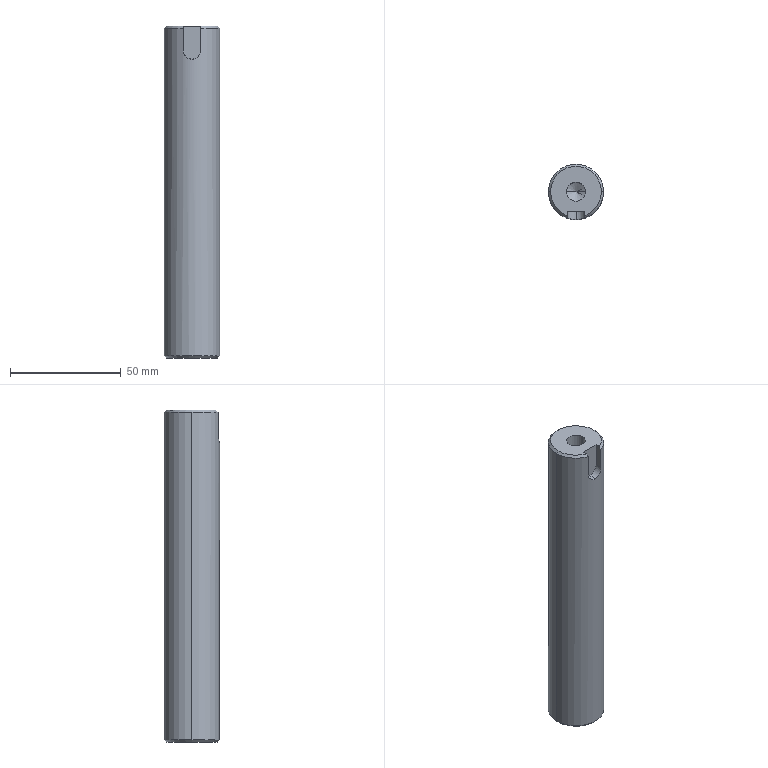Part | SolidWorks | features Chamfer 1, Extrusion 1, Fillet 1, HoleWzd 1, ICE 1 | 1 solid | 18 faces | box 25 x 25 x 150 mm | volume 71725 mm3 | cone 7 | cylinder 6 | plane 5 | commonest cylinder face diameters 8 x2 8.5 x2 25 x2
STEP:
#1=CARTESIAN_POINT('',(-4.25,0.,50.5));
#2=VERTEX_POINT('',#1);
#3=CARTESIAN_POINT('',(4.25,0.,50.5));
#4=VERTEX_POINT('',#3);
#5=CARTESIAN_POINT('',(0.,0.,50.5));
#6=DIRECTION('',(0.,0.,1.));
#7=DIRECTION('',(1.,0.,0.));
#8=AXIS2_PLACEMENT_3D('',#5,#6,#7);
#9=CIRCLE('',#8,4.25);
#10=EDGE_CURVE('',#2,#4,#9,.T.);
#11=ORIENTED_EDGE('',*,*,#10,.F.);
#12=CARTESIAN_POINT('',(-4.25,0.,75.));
#13=VERTEX_POINT('',#12);
#14=CARTESIAN_POINT('',(-4.25,0.,75.));
#15=DIRECTION('',(0.,0.,1.));
#16=VECTOR('',#15,1000.);
#17=LINE('',#14,#16);
#18=EDGE_CURVE('',#2,#13,#17,.T.);
#19=ORIENTED_EDGE('',*,*,#18,.T.);
#20=CARTESIAN_POINT('',(4.25,0.,75.));
#21=VERTEX_POINT('',#20);
#22=CARTESIAN_POINT('',(0.,0.,75.));
#23=DIRECTION('',(0.,0.,1.));
#24=DIRECTION('',(1.,0.,0.));
#25=AXIS2_PLACEMENT_3D('',#22,#23,#24);
#26=CIRCLE('',#25,4.25);
#27=EDGE_CURVE('',#13,#21,#26,.T.);
#28=ORIENTED_EDGE('',*,*,#27,.T.);
#29=CARTESIAN_POINT('',(4.25,0.,75.));
#30=DIRECTION('',(0.,0.,1.));
#31=VECTOR('',#30,1000.);
#32=LINE('',#29,#31);
#33=EDGE_CURVE('',#4,#21,#32,.T.);
#34=ORIENTED_EDGE('',*,*,#33,.F.);
#35=EDGE_LOOP('',(#11,#19,#28,#34));
#36=FACE_OUTER_BOUND('',#35,.T.);
#37=CARTESIAN_POINT('',(0.,0.,75.));
#38=DIRECTION('',(0.,0.,1.));
#39=DIRECTION('',(1.,0.,0.));
#40=AXIS2_PLACEMENT_3D('',#37,#38,#39);
#41=CYLINDRICAL_SURFACE('',#40,4.25);
#42=ADVANCED_FACE('',(#36),#41,.F.);
#43=CARTESIAN_POINT('',(0.,0.,47.946));
#44=VERTEX_POINT('',#43);
#45=CARTESIAN_POINT('',(4.25,0.,50.5));
#46=DIRECTION('',(0.8572,0.,0.515));
#47=VECTOR('',#46,1000.);
#48=LINE('',#45,#47);
#49=EDGE_CURVE('',#44,#4,#48,.T.);
#50=ORIENTED_EDGE('',*,*,#49,.F.);
#51=CARTESIAN_POINT('',(-4.25,0.,50.5));
#52=DIRECTION('',(-0.8572,0.,0.515));
#53=VECTOR('',#52,1000.);
#54=LINE('',#51,#53);
#55=EDGE_CURVE('',#44,#2,#54,.T.);
#56=ORIENTED_EDGE('',*,*,#55,.T.);
#57=ORIENTED_EDGE('',*,*,#10,.T.);
#58=EDGE_LOOP('',(#50,#56,#57));
#59=FACE_OUTER_BOUND('',#58,.T.);
#60=CARTESIAN_POINT('',(0.,0.,50.5));
#61=DIRECTION('',(0.,0.,1.));
#62=DIRECTION('',(1.,0.,0.));
#63=AXIS2_PLACEMENT_3D('',#60,#61,#62);
#64=CONICAL_SURFACE('',#63,4.25,1.03);
#65=ADVANCED_FACE('',(#59),#64,.F.);
#66=CARTESIAN_POINT('',(11.5,0.,75.));
#67=VERTEX_POINT('',#66);
#68=CARTESIAN_POINT('',(-11.5,0.,75.));
#69=VERTEX_POINT('',#68);
#70=CARTESIAN_POINT('',(0.,0.,75.));
#71=DIRECTION('',(0.,0.,1.));
#72=DIRECTION('',(1.,0.,0.));
#73=AXIS2_PLACEMENT_3D('',#70,#71,#72);
#74=CIRCLE('',#73,11.5);
#75=EDGE_CURVE('',#67,#69,#74,.T.);
#76=ORIENTED_EDGE('',*,*,#75,.F.);
#77=CARTESIAN_POINT('',(12.5,0.,74.));
#78=VERTEX_POINT('',#77);
#79=CARTESIAN_POINT('',(11.5,0.,75.));
#80=DIRECTION('',(0.7071,0.,-0.7071));
#81=VECTOR('',#80,1000.);
#82=LINE('',#79,#81);
#83=EDGE_CURVE('',#67,#78,#82,.T.);
#84=ORIENTED_EDGE('',*,*,#83,.T.);
#85=CARTESIAN_POINT('',(-12.5,0.,74.));
#86=VERTEX_POINT('',#85);
#87=CARTESIAN_POINT('',(0.,0.,74.));
#88=DIRECTION('',(0.,0.,-1.));
#89=DIRECTION('',(1.,0.,0.));
#90=AXIS2_PLACEMENT_3D('',#87,#88,#89);
#91=CIRCLE('',#90,12.5);
#92=EDGE_CURVE('',#86,#78,#91,.T.);
#93=ORIENTED_EDGE('',*,*,#92,.F.);
#94=CARTESIAN_POINT('',(-11.5,0.,75.));
#95=DIRECTION('',(-0.7071,0.,-0.7071));
#96=VECTOR('',#95,1000.);
#97=LINE('',#94,#96);
#98=EDGE_CURVE('',#69,#86,#97,.T.);
#99=ORIENTED_EDGE('',*,*,#98,.F.);
#100=EDGE_LOOP('',(#76,#84,#93,#99));
#101=FACE_OUTER_BOUND('',#100,.T.);
#102=CARTESIAN_POINT('',(0.,0.,75.));
#103=DIRECTION('',(0.,0.,-1.));
#104=DIRECTION('',(-1.,0.,0.));
#105=AXIS2_PLACEMENT_3D('',#102,#103,#104);
#106=CONICAL_SURFACE('',#105,11.5,0.7854);
#107=ADVANCED_FACE('',(#101),#106,.T.);
#108=CARTESIAN_POINT('',(-4.,-10.782,75.));
#109=VERTEX_POINT('',#108);
#110=CARTESIAN_POINT('',(0.,0.,75.));
#111=DIRECTION('',(0.,0.,1.));
#112=DIRECTION('',(1.,0.,0.));
#113=AXIS2_PLACEMENT_3D('',#110,#111,#112);
#114=CIRCLE('',#113,11.5);
#115=EDGE_CURVE('',#69,#109,#114,.T.);
#116=ORIENTED_EDGE('',*,*,#115,.F.);
#117=ORIENTED_EDGE('',*,*,#98,.T.);
#118=CARTESIAN_POINT('',(-4.,-11.843,74.));
#119=VERTEX_POINT('',#118);
#120=CARTESIAN_POINT('',(0.,0.,74.));
#121=DIRECTION('',(0.,0.,-1.));
#122=DIRECTION('',(1.,0.,0.));
#123=AXIS2_PLACEMENT_3D('',#120,#121,#122);
#124=CIRCLE('',#123,12.5);
#125=EDGE_CURVE('',#119,#86,#124,.T.);
#126=ORIENTED_EDGE('',*,*,#125,.F.);
#127=CARTESIAN_POINT('',(-4.,-10.782,75.));
#128=CARTESIAN_POINT('',(-4.,-11.136,74.668));
#129=CARTESIAN_POINT('',(-4.,-11.49,74.334));
#130=CARTESIAN_POINT('',(-4.,-11.843,74.));
#131=B_SPLINE_CURVE_WITH_KNOTS('',3,(#127,#128,#129,#130),.UNSPECIFIED.,.F.,.F.,(4,4),(0.005716,0.007174),.UNSPECIFIED.);
#132=EDGE_CURVE('',#109,#119,#131,.T.);
#133=ORIENTED_EDGE('',*,*,#132,.F.);
#134=EDGE_LOOP('',(#116,#117,#126,#133));
#135=FACE_OUTER_BOUND('',#134,.T.);
#136=CARTESIAN_POINT('',(0.,0.,75.));
#137=DIRECTION('',(0.,0.,-1.));
#138=DIRECTION('',(-1.,0.,0.));
#139=AXIS2_PLACEMENT_3D('',#136,#137,#138);
#140=CONICAL_SURFACE('',#139,11.5,0.7854);
#141=ADVANCED_FACE('',(#135),#140,.T.);
#142=CARTESIAN_POINT('',(-11.5,0.,-75.));
#143=VERTEX_POINT('',#142);
#144=CARTESIAN_POINT('',(11.5,0.,-75.));
#145=VERTEX_POINT('',#144);
#146=CARTESIAN_POINT('',(0.,0.,-75.));
#147=DIRECTION('',(0.,0.,-1.));
#148=DIRECTION('',(1.,0.,0.));
#149=AXIS2_PLACEMENT_3D('',#146,#147,#148);
#150=CIRCLE('',#149,11.5);
#151=EDGE_CURVE('',#143,#145,#150,.T.);
#152=ORIENTED_EDGE('',*,*,#151,.F.);
#153=CARTESIAN_POINT('',(-12.5,0.,-74.));
#154=VERTEX_POINT('',#153);
#155=CARTESIAN_POINT('',(-12.5,0.,-74.));
#156=DIRECTION('',(-0.7071,0.,0.7071));
#157=VECTOR('',#156,1000.);
#158=LINE('',#155,#157);
#159=EDGE_CURVE('',#143,#154,#158,.T.);
#160=ORIENTED_EDGE('',*,*,#159,.T.);
#161=CARTESIAN_POINT('',(12.5,0.,-74.));
#162=VERTEX_POINT('',#161);
#163=CARTESIAN_POINT('',(0.,0.,-74.));
#164=DIRECTION('',(0.,0.,1.));
#165=DIRECTION('',(1.,0.,0.));
#166=AXIS2_PLACEMENT_3D('',#163,#164,#165);
#167=CIRCLE('',#166,12.5);
#168=EDGE_CURVE('',#162,#154,#167,.T.);
#169=ORIENTED_EDGE('',*,*,#168,.F.);
#170=CARTESIAN_POINT('',(12.5,0.,-74.));
#171=DIRECTION('',(0.7071,0.,0.7071));
#172=VECTOR('',#171,1000.);
#173=LINE('',#170,#172);
#174=EDGE_CURVE('',#145,#162,#173,.T.);
#175=ORIENTED_EDGE('',*,*,#174,.F.);
#176=EDGE_LOOP('',(#152,#160,#169,#175));
#177=FACE_OUTER_BOUND('',#176,.T.);
#178=CARTESIAN_POINT('',(0.,0.,-74.));
#179=DIRECTION('',(0.,0.,1.));
#180=DIRECTION('',(1.,0.,0.));
#181=AXIS2_PLACEMENT_3D('',#178,#179,#180);
#182=CONICAL_SURFACE('',#181,12.5,0.7854);
#183=ADVANCED_FACE('',(#177),#182,.T.);
#184=ORIENTED_EDGE('',*,*,#92,.T.);
#185=CARTESIAN_POINT('',(12.5,0.,75.));
#186=DIRECTION('',(0.,0.,-1.));
#187=VECTOR('',#186,1000.);
#188=LINE('',#185,#187);
#189=EDGE_CURVE('',#78,#162,#188,.T.);
#190=ORIENTED_EDGE('',*,*,#189,.T.);
#191=ORIENTED_EDGE('',*,*,#168,.T.);
#192=CARTESIAN_POINT('',(-12.5,0.,75.));
#193=DIRECTION('',(0.,0.,-1.));
#194=VECTOR('',#193,1000.);
#195=LINE('',#192,#194);
#196=EDGE_CURVE('',#86,#154,#195,.T.);
#197=ORIENTED_EDGE('',*,*,#196,.F.);
#198=EDGE_LOOP('',(#184,#190,#191,#197));
#199=FACE_OUTER_BOUND('',#198,.T.);
#200=CARTESIAN_POINT('',(0.,0.,75.));
#201=DIRECTION('',(0.,0.,-1.));
#202=DIRECTION('',(-1.,0.,0.));
#203=AXIS2_PLACEMENT_3D('',#200,#201,#202);
#204=CYLINDRICAL_SURFACE('',#203,12.5);
#205=ADVANCED_FACE('',(#199),#204,.T.);
#206=ORIENTED_EDGE('',*,*,#189,.F.);
#207=CARTESIAN_POINT('',(4.,-11.843,74.));
#208=VERTEX_POINT('',#207);
#209=CARTESIAN_POINT('',(0.,0.,74.));
#210=DIRECTION('',(0.,0.,-1.));
#211=DIRECTION('',(1.,0.,0.));
#212=AXIS2_PLACEMENT_3D('',#209,#210,#211);
#213=CIRCLE('',#212,12.5);
#214=EDGE_CURVE('',#78,#208,#213,.T.);
#215=ORIENTED_EDGE('',*,*,#214,.T.);
#216=CARTESIAN_POINT('',(4.,-11.843,64.));
#217=VERTEX_POINT('',#216);
#218=CARTESIAN_POINT('',(4.,-11.843,75.));
#219=DIRECTION('',(0.,0.,-1.));
#220=VECTOR('',#219,1000.);
#221=LINE('',#218,#220);
#222=EDGE_CURVE('',#208,#217,#221,.T.);
#223=ORIENTED_EDGE('',*,*,#222,.T.);
#224=CARTESIAN_POINT('',(0.,-12.5,60.));
#225=VERTEX_POINT('',#224);
#226=CARTESIAN_POINT('',(4.,-11.843,64.));
#227=CARTESIAN_POINT('',(4.,-11.843,63.734));
#228=CARTESIAN_POINT('',(3.974,-11.852,63.473));
#229=CARTESIAN_POINT('',(3.871,-11.886,62.96));
#230=CARTESIAN_POINT('',(3.794,-11.911,62.705));
#231=CARTESIAN_POINT('',(3.592,-11.973,62.221));
#232=CARTESIAN_POINT('',(3.47,-12.01,61.993));
#233=CARTESIAN_POINT('',(3.18,-12.09,61.559));
#234=CARTESIAN_POINT('',(3.012,-12.133,61.356));
#235=CARTESIAN_POINT('',(2.646,-12.218,60.989));
#236=CARTESIAN_POINT('',(2.446,-12.26,60.824));
#237=CARTESIAN_POINT('',(2.01,-12.339,60.532));
#238=CARTESIAN_POINT('',(1.78,-12.375,60.409));
#239=CARTESIAN_POINT('',(1.3,-12.435,60.208));
#240=CARTESIAN_POINT('',(1.047,-12.459,60.13));
#241=CARTESIAN_POINT('',(0.5285,-12.492,60.026));
#242=CARTESIAN_POINT('',(0.266,-12.5,60.));
#243=CARTESIAN_POINT('',(0.,-12.5,60.));
#244=B_SPLINE_CURVE_WITH_KNOTS('',3,(#226,#227,#228,#229,#230,#231,#232,#233,#234,#235,#236,#237,#238,#239,#240,#241,#242,#243),.UNSPECIFIED.,.F.,.F.,(4,2,2,2,2,2,2,2,4),(0.,0.0007863,0.001573,0.002359,0.003145,0.003931,0.004718,0.005504,0.00629),.UNSPECIFIED.);
#245=EDGE_CURVE('',#217,#225,#244,.T.);
#246=ORIENTED_EDGE('',*,*,#245,.T.);
#247=CARTESIAN_POINT('',(-4.,-11.843,64.));
#248=VERTEX_POINT('',#247);
#249=CARTESIAN_POINT('',(0.,-12.5,60.));
#250=CARTESIAN_POINT('',(-0.266,-12.5,60.));
#251=CARTESIAN_POINT('',(-0.5272,-12.492,60.026));
#252=CARTESIAN_POINT('',(-1.041,-12.459,60.129));
#253=CARTESIAN_POINT('',(-1.296,-12.435,60.207));
#254=CARTESIAN_POINT('',(-1.779,-12.375,60.408));
#255=CARTESIAN_POINT('',(-2.008,-12.34,60.531));
#256=CARTESIAN_POINT('',(-2.441,-12.261,60.821));
#257=CARTESIAN_POINT('',(-2.645,-12.218,60.988));
#258=CARTESIAN_POINT('',(-3.011,-12.133,61.354));
#259=CARTESIAN_POINT('',(-3.176,-12.091,61.554));
#260=CARTESIAN_POINT('',(-3.469,-12.01,61.991));
#261=CARTESIAN_POINT('',(-3.592,-11.973,62.22));
#262=CARTESIAN_POINT('',(-3.792,-11.911,62.7));
#263=CARTESIAN_POINT('',(-3.87,-11.886,62.954));
#264=CARTESIAN_POINT('',(-3.974,-11.852,63.472));
#265=CARTESIAN_POINT('',(-4.,-11.843,63.734));
#266=CARTESIAN_POINT('',(-4.,-11.843,64.));
#267=B_SPLINE_CURVE_WITH_KNOTS('',3,(#249,#250,#251,#252,#253,#254,#255,#256,#257,#258,#259,#260,#261,#262,#263,#264,#265,#266),.UNSPECIFIED.,.F.,.F.,(4,2,2,2,2,2,2,2,4),(0.,0.0007863,0.001573,0.002359,0.003145,0.003932,0.004718,0.005504,0.00629),.UNSPECIFIED.);
#268=EDGE_CURVE('',#225,#248,#267,.T.);
#269=ORIENTED_EDGE('',*,*,#268,.T.);
#270=CARTESIAN_POINT('',(-4.,-11.843,75.));
#271=DIRECTION('',(0.,0.,1.));
#272=VECTOR('',#271,1000.);
#273=LINE('',#270,#272);
#274=EDGE_CURVE('',#248,#119,#273,.T.);
#275=ORIENTED_EDGE('',*,*,#274,.T.);
#276=ORIENTED_EDGE('',*,*,#125,.T.);
#277=ORIENTED_EDGE('',*,*,#196,.T.);
#278=CARTESIAN_POINT('',(0.,0.,-74.));
#279=DIRECTION('',(0.,0.,1.));
#280=DIRECTION('',(1.,0.,0.));
#281=AXIS2_PLACEMENT_3D('',#278,#279,#280);
#282=CIRCLE('',#281,12.5);
#283=EDGE_CURVE('',#154,#162,#282,.T.);
#284=ORIENTED_EDGE('',*,*,#283,.T.);
#285=EDGE_LOOP('',(#206,#215,#223,#246,#269,#275,#276,#277,#284));
#286=FACE_OUTER_BOUND('',#285,.T.);
#287=CARTESIAN_POINT('',(0.,0.,75.));
#288=DIRECTION('',(0.,0.,-1.));
#289=DIRECTION('',(-1.,0.,0.));
#290=AXIS2_PLACEMENT_3D('',#287,#288,#289);
#291=CYLINDRICAL_SURFACE('',#290,12.5);
#292=ADVANCED_FACE('',(#286),#291,.T.);
#293=CARTESIAN_POINT('',(-4.,-8.8,75.));
#294=VERTEX_POINT('',#293);
#295=CARTESIAN_POINT('',(-4.,-18.8,75.));
#296=DIRECTION('',(0.,1.,0.));
#297=VECTOR('',#296,1000.);
#298=LINE('',#295,#297);
#299=EDGE_CURVE('',#109,#294,#298,.T.);
#300=ORIENTED_EDGE('',*,*,#299,.T.);
#301=CARTESIAN_POINT('',(4.,-8.8,75.));
#302=VERTEX_POINT('',#301);
#303=CARTESIAN_POINT('',(-4.,-8.8,75.));
#304=DIRECTION('',(1.,0.,0.));
#305=VECTOR('',#304,1000.);
#306=LINE('',#303,#305);
#307=EDGE_CURVE('',#294,#302,#306,.T.);
#308=ORIENTED_EDGE('',*,*,#307,.T.);
#309=CARTESIAN_POINT('',(4.,-10.782,75.));
#310=VERTEX_POINT('',#309);
#311=CARTESIAN_POINT('',(4.,-18.8,75.));
#312=DIRECTION('',(0.,1.,0.));
#313=VECTOR('',#312,1000.);
#314=LINE('',#311,#313);
#315=EDGE_CURVE('',#310,#302,#314,.T.);
#316=ORIENTED_EDGE('',*,*,#315,.F.);
#317=CARTESIAN_POINT('',(0.,0.,75.));
#318=DIRECTION('',(0.,0.,1.));
#319=DIRECTION('',(1.,0.,0.));
#320=AXIS2_PLACEMENT_3D('',#317,#318,#319);
#321=CIRCLE('',#320,11.5);
#322=EDGE_CURVE('',#310,#67,#321,.T.);
#323=ORIENTED_EDGE('',*,*,#322,.T.);
#324=ORIENTED_EDGE('',*,*,#75,.T.);
#325=ORIENTED_EDGE('',*,*,#115,.T.);
#326=EDGE_LOOP('',(#300,#308,#316,#323,#324,#325));
#327=FACE_OUTER_BOUND('',#326,.T.);
#328=CARTESIAN_POINT('',(0.,0.,75.));
#329=DIRECTION('',(0.,0.,1.));
#330=DIRECTION('',(1.,0.,0.));
#331=AXIS2_PLACEMENT_3D('',#328,#329,#330);
#332=CIRCLE('',#331,4.25);
#333=EDGE_CURVE('',#21,#13,#332,.T.);
#334=ORIENTED_EDGE('',*,*,#333,.F.);
#335=ORIENTED_EDGE('',*,*,#27,.F.);
#336=EDGE_LOOP('',(#334,#335));
#337=FACE_BOUND('',#336,.T.);
#338=CARTESIAN_POINT('',(0.,0.,75.));
#339=DIRECTION('',(0.,0.,1.));
#340=DIRECTION('',(1.,0.,0.));
#341=AXIS2_PLACEMENT_3D('',#338,#339,#340);
#342=PLANE('',#341);
#343=ADVANCED_FACE('',(#327,#337),#342,.T.);
#344=CARTESIAN_POINT('',(0.,0.,-75.));
#345=DIRECTION('',(0.,0.,-1.));
#346=DIRECTION('',(1.,0.,0.));
#347=AXIS2_PLACEMENT_3D('',#344,#345,#346);
#348=CIRCLE('',#347,11.5);
#349=EDGE_CURVE('',#145,#143,#348,.T.);
#350=ORIENTED_EDGE('',*,*,#349,.T.);
#351=ORIENTED_EDGE('',*,*,#151,.T.);
#352=EDGE_LOOP('',(#350,#351));
#353=FACE_OUTER_BOUND('',#352,.T.);
#354=CARTESIAN_POINT('',(0.,0.,-75.));
#355=DIRECTION('',(0.,0.,1.));
#356=DIRECTION('',(1.,0.,0.));
#357=AXIS2_PLACEMENT_3D('',#354,#355,#356);
#358=PLANE('',#357);
#359=ADVANCED_FACE('',(#353),#358,.F.);
#360=ORIENTED_EDGE('',*,*,#159,.F.);
#361=ORIENTED_EDGE('',*,*,#349,.F.);
#362=ORIENTED_EDGE('',*,*,#174,.T.);
#363=ORIENTED_EDGE('',*,*,#283,.F.);
#364=EDGE_LOOP('',(#360,#361,#362,#363));
#365=FACE_OUTER_BOUND('',#364,.T.);
#366=CARTESIAN_POINT('',(0.,0.,-74.));
#367=DIRECTION('',(0.,0.,1.));
#368=DIRECTION('',(1.,0.,0.));
#369=AXIS2_PLACEMENT_3D('',#366,#367,#368);
#370=CONICAL_SURFACE('',#369,12.5,0.7854);
#371=ADVANCED_FACE('',(#365),#370,.T.);
#372=ORIENTED_EDGE('',*,*,#83,.F.);
#373=ORIENTED_EDGE('',*,*,#322,.F.);
#374=CARTESIAN_POINT('',(4.,-11.843,74.));
#375=CARTESIAN_POINT('',(4.,-11.49,74.334));
#376=CARTESIAN_POINT('',(4.,-11.136,74.668));
#377=CARTESIAN_POINT('',(4.,-10.782,75.));
#378=B_SPLINE_CURVE_WITH_KNOTS('',3,(#374,#375,#376,#377),.UNSPECIFIED.,.F.,.F.,(4,4),(0.005534,0.006992),.UNSPECIFIED.);
#379=EDGE_CURVE('',#208,#310,#378,.T.);
#380=ORIENTED_EDGE('',*,*,#379,.F.);
#381=ORIENTED_EDGE('',*,*,#214,.F.);
#382=EDGE_LOOP('',(#372,#373,#380,#381));
#383=FACE_OUTER_BOUND('',#382,.T.);
#384=CARTESIAN_POINT('',(0.,0.,75.));
#385=DIRECTION('',(0.,0.,-1.));
#386=DIRECTION('',(-1.,0.,0.));
#387=AXIS2_PLACEMENT_3D('',#384,#385,#386);
#388=CONICAL_SURFACE('',#387,11.5,0.7854);
#389=ADVANCED_FACE('',(#383),#388,.T.);
#390=ORIENTED_EDGE('',*,*,#55,.F.);
#391=ORIENTED_EDGE('',*,*,#49,.T.);
#392=CARTESIAN_POINT('',(0.,0.,50.5));
#393=DIRECTION('',(0.,0.,1.));
#394=DIRECTION('',(1.,0.,0.));
#395=AXIS2_PLACEMENT_3D('',#392,#393,#394);
#396=CIRCLE('',#395,4.25);
#397=EDGE_CURVE('',#4,#2,#396,.T.);
#398=ORIENTED_EDGE('',*,*,#397,.T.);
#399=EDGE_LOOP('',(#390,#391,#398));
#400=FACE_OUTER_BOUND('',#399,.T.);
#401=CARTESIAN_POINT('',(0.,0.,50.5));
#402=DIRECTION('',(0.,0.,1.));
#403=DIRECTION('',(1.,0.,0.));
#404=AXIS2_PLACEMENT_3D('',#401,#402,#403);
#405=CONICAL_SURFACE('',#404,4.25,1.03);
#406=ADVANCED_FACE('',(#400),#405,.F.);
#407=ORIENTED_EDGE('',*,*,#18,.F.);
#408=ORIENTED_EDGE('',*,*,#397,.F.);
#409=ORIENTED_EDGE('',*,*,#33,.T.);
#410=ORIENTED_EDGE('',*,*,#333,.T.);
#411=EDGE_LOOP('',(#407,#408,#409,#410));
#412=FACE_OUTER_BOUND('',#411,.T.);
#413=CARTESIAN_POINT('',(0.,0.,75.));
#414=DIRECTION('',(0.,0.,1.));
#415=DIRECTION('',(1.,0.,0.));
#416=AXIS2_PLACEMENT_3D('',#413,#414,#415);
#417=CYLINDRICAL_SURFACE('',#416,4.25);
#418=ADVANCED_FACE('',(#412),#417,.F.);
#419=ORIENTED_EDGE('',*,*,#274,.F.);
#420=CARTESIAN_POINT('',(-4.,-8.8,64.));
#421=VERTEX_POINT('',#420);
#422=CARTESIAN_POINT('',(-4.,-8.8,64.));
#423=DIRECTION('',(0.,1.,0.));
#424=VECTOR('',#423,1000.);
#425=LINE('',#422,#424);
#426=EDGE_CURVE('',#248,#421,#425,.T.);
#427=ORIENTED_EDGE('',*,*,#426,.T.);
#428=CARTESIAN_POINT('',(-4.,-8.8,75.));
#429=DIRECTION('',(0.,0.,1.));
#430=VECTOR('',#429,1000.);
#431=LINE('',#428,#430);
#432=EDGE_CURVE('',#421,#294,#431,.T.);
#433=ORIENTED_EDGE('',*,*,#432,.T.);
#434=ORIENTED_EDGE('',*,*,#299,.F.);
#435=ORIENTED_EDGE('',*,*,#132,.T.);
#436=EDGE_LOOP('',(#419,#427,#433,#434,#435));
#437=FACE_OUTER_BOUND('',#436,.T.);
#438=CARTESIAN_POINT('',(-4.,-18.8,75.));
#439=DIRECTION('',(-1.,0.,0.));
#440=DIRECTION('',(0.,0.,1.));
#441=AXIS2_PLACEMENT_3D('',#438,#439,#440);
#442=PLANE('',#441);
#443=ADVANCED_FACE('',(#437),#442,.F.);
#444=CARTESIAN_POINT('',(4.,-8.8,64.));
#445=VERTEX_POINT('',#444);
#446=CARTESIAN_POINT('',(4.,-8.8,75.));
#447=DIRECTION('',(0.,0.,-1.));
#448=VECTOR('',#447,1000.);
#449=LINE('',#446,#448);
#450=EDGE_CURVE('',#302,#445,#449,.T.);
#451=ORIENTED_EDGE('',*,*,#450,.T.);
#452=CARTESIAN_POINT('',(4.,-11.843,64.));
#453=DIRECTION('',(0.,-1.,0.));
#454=VECTOR('',#453,1000.);
#455=LINE('',#452,#454);
#456=EDGE_CURVE('',#445,#217,#455,.T.);
#457=ORIENTED_EDGE('',*,*,#456,.T.);
#458=ORIENTED_EDGE('',*,*,#222,.F.);
#459=ORIENTED_EDGE('',*,*,#379,.T.);
#460=ORIENTED_EDGE('',*,*,#315,.T.);
#461=EDGE_LOOP('',(#451,#457,#458,#459,#460));
#462=FACE_OUTER_BOUND('',#461,.T.);
#463=CARTESIAN_POINT('',(4.,-18.8,75.));
#464=DIRECTION('',(1.,0.,0.));
#465=DIRECTION('',(0.,0.,-1.));
#466=AXIS2_PLACEMENT_3D('',#463,#464,#465);
#467=PLANE('',#466);
#468=ADVANCED_FACE('',(#462),#467,.F.);
#469=CARTESIAN_POINT('',(0.,-8.8,60.));
#470=VERTEX_POINT('',#469);
#471=CARTESIAN_POINT('',(0.,-8.8,64.));
#472=DIRECTION('',(0.,-1.,0.));
#473=DIRECTION('',(0.,0.,-1.));
#474=AXIS2_PLACEMENT_3D('',#471,#472,#473);
#475=CIRCLE('',#474,4.);
#476=EDGE_CURVE('',#421,#470,#475,.T.);
#477=ORIENTED_EDGE('',*,*,#476,.T.);
#478=CARTESIAN_POINT('',(0.,-8.8,64.));
#479=DIRECTION('',(0.,-1.,0.));
#480=DIRECTION('',(0.,0.,-1.));
#481=AXIS2_PLACEMENT_3D('',#478,#479,#480);
#482=CIRCLE('',#481,4.);
#483=EDGE_CURVE('',#470,#445,#482,.T.);
#484=ORIENTED_EDGE('',*,*,#483,.T.);
#485=ORIENTED_EDGE('',*,*,#450,.F.);
#486=ORIENTED_EDGE('',*,*,#307,.F.);
#487=ORIENTED_EDGE('',*,*,#432,.F.);
#488=EDGE_LOOP('',(#477,#484,#485,#486,#487));
#489=FACE_OUTER_BOUND('',#488,.T.);
#490=CARTESIAN_POINT('',(0.,-8.8,0.));
#491=DIRECTION('',(0.,-1.,0.));
#492=DIRECTION('',(0.,0.,-1.));
#493=AXIS2_PLACEMENT_3D('',#490,#491,#492);
#494=PLANE('',#493);
#495=ADVANCED_FACE('',(#489),#494,.T.);
#496=ORIENTED_EDGE('',*,*,#426,.F.);
#497=ORIENTED_EDGE('',*,*,#268,.F.);
#498=CARTESIAN_POINT('',(0.,-11.843,60.));
#499=DIRECTION('',(0.,-1.,0.));
#500=VECTOR('',#499,1000.);
#501=LINE('',#498,#500);
#502=EDGE_CURVE('',#470,#225,#501,.T.);
#503=ORIENTED_EDGE('',*,*,#502,.F.);
#504=ORIENTED_EDGE('',*,*,#476,.F.);
#505=EDGE_LOOP('',(#496,#497,#503,#504));
#506=FACE_OUTER_BOUND('',#505,.T.);
#507=CARTESIAN_POINT('',(0.,-18.8,64.));
#508=DIRECTION('',(0.,-1.,0.));
#509=DIRECTION('',(0.,0.,-1.));
#510=AXIS2_PLACEMENT_3D('',#507,#508,#509);
#511=CYLINDRICAL_SURFACE('',#510,4.);
#512=ADVANCED_FACE('',(#506),#511,.F.);
#513=ORIENTED_EDGE('',*,*,#245,.F.);
#514=ORIENTED_EDGE('',*,*,#456,.F.);
#515=ORIENTED_EDGE('',*,*,#483,.F.);
#516=ORIENTED_EDGE('',*,*,#502,.T.);
#517=EDGE_LOOP('',(#513,#514,#515,#516));
#518=FACE_OUTER_BOUND('',#517,.T.);
#519=CARTESIAN_POINT('',(0.,-18.8,64.));
#520=DIRECTION('',(0.,-1.,0.));
#521=DIRECTION('',(0.,0.,-1.));
#522=AXIS2_PLACEMENT_3D('',#519,#520,#521);
#523=CYLINDRICAL_SURFACE('',#522,4.);
#524=ADVANCED_FACE('',(#518),#523,.F.);
#525=CLOSED_SHELL('',(#42,#65,#107,#141,#183,#205,#292,#343,#359,#371,#389,#406,#418,#443,#468,#495,#512,#524));
#526=MANIFOLD_SOLID_BREP('',#525);
#527=CARTESIAN_POINT('',(0.,0.,0.));
#528=DIRECTION('',(0.,0.,1.));
#529=DIRECTION('',(1.,0.,0.));
#530=AXIS2_PLACEMENT_3D('',#527,#528,#529);
#531=(LENGTH_UNIT()NAMED_UNIT(*)SI_UNIT(.MILLI.,.METRE.));
#532=UNCERTAINTY_MEASURE_WITH_UNIT(LENGTH_MEASURE(0.00001),#531,'','');
#533=(NAMED_UNIT(*)PLANE_ANGLE_UNIT()SI_UNIT($,.RADIAN.));
#534=(NAMED_UNIT(*)SI_UNIT($,.STERADIAN.)SOLID_ANGLE_UNIT());
#535=(GEOMETRIC_REPRESENTATION_CONTEXT(3)GLOBAL_UNCERTAINTY_ASSIGNED_CONTEXT((#532))GLOBAL_UNIT_ASSIGNED_CONTEXT((#531,#533,#534))REPRESENTATION_CONTEXT('',''));
#536=ADVANCED_BREP_SHAPE_REPRESENTATION('',(#526,#530),#535);